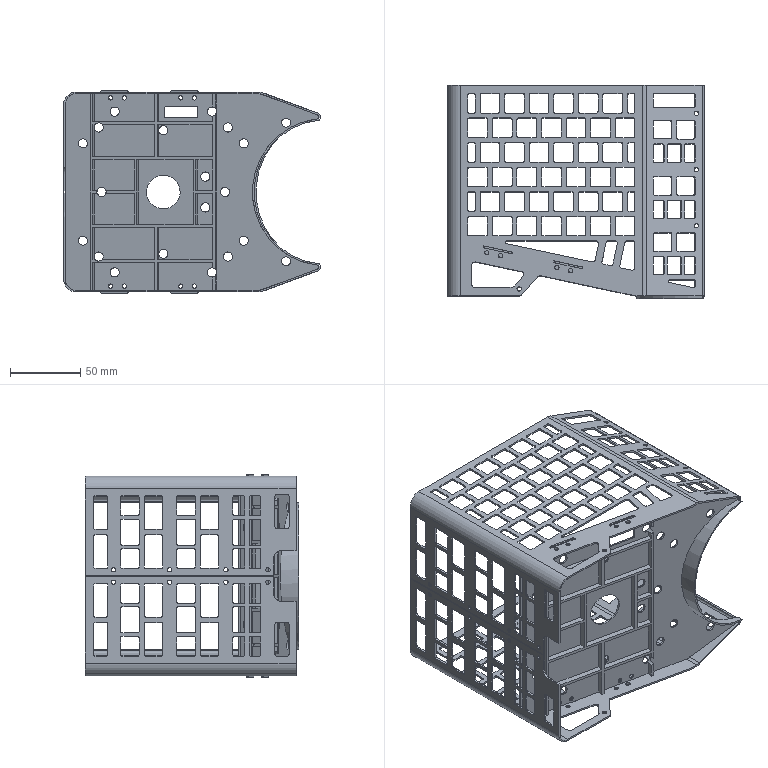Part | SolidWorks | features Fillet 17, ICE 10, Extrusion 1, MirrorPattern 1 | 5 solids | 1672 faces | box 182.976 x 151.8 x 144 mm | volume 82758 mm3 | plane 837 | cylinder 755 | spline 80 | commonest cylinder face diameters 2 x584 3.1 x64 6.5 x40 3 x34 6 x12 4 x8